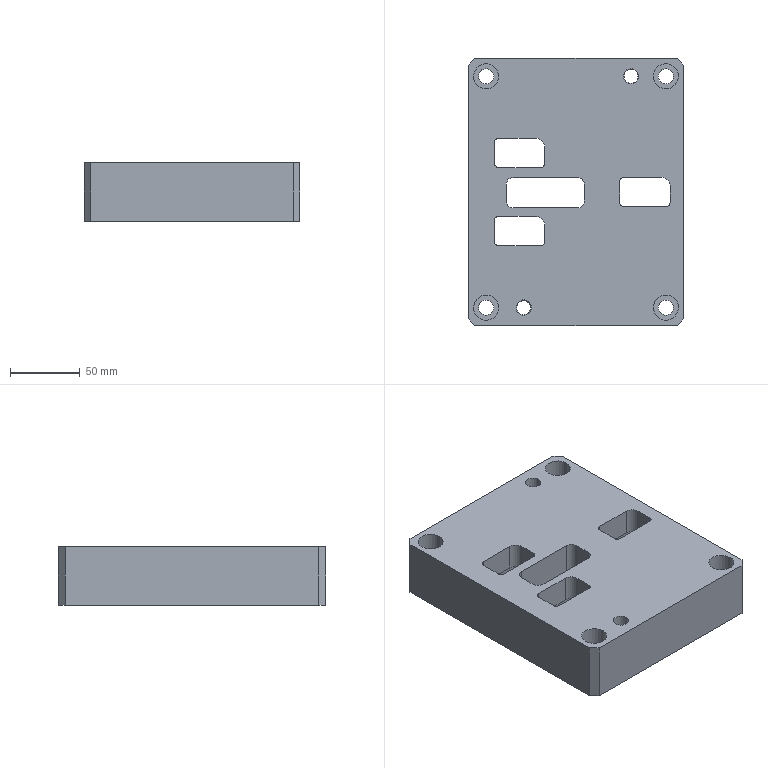Part | CATIA | 1 solid | 101 faces | box 155 x 192 x 42 mm | volume 1025287 mm3 | cylinder 52 | plane 45 | cone 4 | commonest cylinder face diameters 10 x20 11 x12 6 x9 18 x8 12 x3